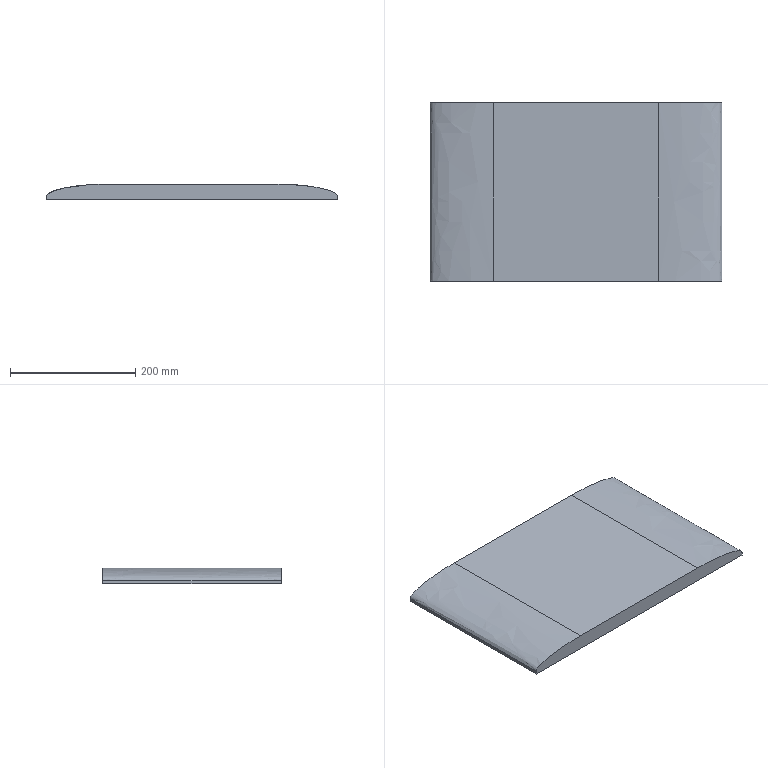Part | SolidWorks | features Fillet 2, Extrusion 1 | 1 solid | 8 faces | box 465 x 285 x 25.029 mm | volume 3079068 mm3 | plane 6 | spline 2
STEP:
#1=CARTESIAN_POINT('',(-232.5,-142.5,5.029));
#2=VERTEX_POINT('',#1);
#3=CARTESIAN_POINT('',(-232.5,-142.5,0.));
#4=VERTEX_POINT('',#3);
#5=CARTESIAN_POINT('',(-232.5,-142.5,25.029));
#6=DIRECTION('',(0.,0.,-1.));
#7=VECTOR('',#6,1000.);
#8=LINE('',#5,#7);
#9=EDGE_CURVE('',#2,#4,#8,.T.);
#10=ORIENTED_EDGE('',*,*,#9,.F.);
#11=CARTESIAN_POINT('',(-232.5,142.5,5.029));
#12=VERTEX_POINT('',#11);
#13=CARTESIAN_POINT('',(-232.5,-142.5,5.029));
#14=CARTESIAN_POINT('',(-232.5,-47.5,5.029));
#15=CARTESIAN_POINT('',(-232.5,47.5,5.029));
#16=CARTESIAN_POINT('',(-232.5,142.5,5.029));
#17=B_SPLINE_CURVE_WITH_KNOTS('',3,(#13,#14,#15,#16),.UNSPECIFIED.,.F.,.F.,(4,4),(0.,1.),.UNSPECIFIED.);
#18=EDGE_CURVE('',#2,#12,#17,.T.);
#19=ORIENTED_EDGE('',*,*,#18,.T.);
#20=CARTESIAN_POINT('',(-232.5,142.5,0.));
#21=VERTEX_POINT('',#20);
#22=CARTESIAN_POINT('',(-232.5,142.5,25.029));
#23=DIRECTION('',(0.,0.,-1.));
#24=VECTOR('',#23,1000.);
#25=LINE('',#22,#24);
#26=EDGE_CURVE('',#12,#21,#25,.T.);
#27=ORIENTED_EDGE('',*,*,#26,.T.);
#28=CARTESIAN_POINT('',(-232.5,-142.5,0.));
#29=DIRECTION('',(0.,-1.,0.));
#30=VECTOR('',#29,1000.);
#31=LINE('',#28,#30);
#32=EDGE_CURVE('',#21,#4,#31,.T.);
#33=ORIENTED_EDGE('',*,*,#32,.T.);
#34=EDGE_LOOP('',(#10,#19,#27,#33));
#35=FACE_OUTER_BOUND('',#34,.T.);
#36=CARTESIAN_POINT('',(-232.5,-142.5,25.029));
#37=DIRECTION('',(1.,0.,0.));
#38=DIRECTION('',(0.,0.,-1.));
#39=AXIS2_PLACEMENT_3D('',#36,#37,#38);
#40=PLANE('',#39);
#41=ADVANCED_FACE('',(#35),#40,.F.);
#42=CARTESIAN_POINT('',(232.5,-142.5,5.029));
#43=VERTEX_POINT('',#42);
#44=CARTESIAN_POINT('',(232.5,-142.5,0.));
#45=VERTEX_POINT('',#44);
#46=CARTESIAN_POINT('',(232.5,-142.5,25.029));
#47=DIRECTION('',(0.,0.,-1.));
#48=VECTOR('',#47,1000.);
#49=LINE('',#46,#48);
#50=EDGE_CURVE('',#43,#45,#49,.T.);
#51=ORIENTED_EDGE('',*,*,#50,.F.);
#52=CARTESIAN_POINT('',(132.5,-142.5,25.029));
#53=VERTEX_POINT('',#52);
#54=CARTESIAN_POINT('',(232.5,-142.5,5.029));
#55=CARTESIAN_POINT('',(232.5,-142.5,5.932));
#56=CARTESIAN_POINT('',(232.05,-142.5,7.274));
#57=CARTESIAN_POINT('',(230.736,-142.5,8.819));
#58=CARTESIAN_POINT('',(229.882,-142.5,9.586));
#59=CARTESIAN_POINT('',(229.405,-142.5,9.968));
#60=CARTESIAN_POINT('',(229.155,-142.5,10.159));
#61=CARTESIAN_POINT('',(229.027,-142.5,10.254));
#62=CARTESIAN_POINT('',(228.962,-142.5,10.302));
#63=CARTESIAN_POINT('',(228.929,-142.5,10.325));
#64=CARTESIAN_POINT('',(228.915,-142.5,10.336));
#65=CARTESIAN_POINT('',(228.906,-142.5,10.342));
#66=CARTESIAN_POINT('',(228.899,-142.5,10.347));
#67=CARTESIAN_POINT('',(228.151,-142.5,10.889));
#68=CARTESIAN_POINT('',(226.869,-142.5,11.687));
#69=CARTESIAN_POINT('',(225.083,-142.5,12.596));
#70=CARTESIAN_POINT('',(224.118,-142.5,13.046));
#71=CARTESIAN_POINT('',(223.618,-142.5,13.269));
#72=CARTESIAN_POINT('',(223.363,-142.5,13.381));
#73=CARTESIAN_POINT('',(223.234,-142.5,13.436));
#74=CARTESIAN_POINT('',(223.17,-142.5,13.464));
#75=CARTESIAN_POINT('',(223.137,-142.5,13.478));
#76=CARTESIAN_POINT('',(223.124,-142.5,13.484));
#77=CARTESIAN_POINT('',(223.114,-142.5,13.488));
#78=CARTESIAN_POINT('',(223.108,-142.5,13.491));
#79=CARTESIAN_POINT('',(221.419,-142.5,14.214));
#80=CARTESIAN_POINT('',(218.59,-142.5,15.259));
#81=CARTESIAN_POINT('',(214.761,-142.5,16.413));
#82=CARTESIAN_POINT('',(212.714,-142.5,16.974));
#83=CARTESIAN_POINT('',(211.658,-142.5,17.251));
#84=CARTESIAN_POINT('',(211.122,-142.5,17.388));
#85=CARTESIAN_POINT('',(210.852,-142.5,17.456));
#86=CARTESIAN_POINT('',(210.716,-142.5,17.49));
#87=CARTESIAN_POINT('',(210.648,-142.5,17.507));
#88=CARTESIAN_POINT('',(210.614,-142.5,17.516));
#89=CARTESIAN_POINT('',(210.599,-142.5,17.519));
#90=CARTESIAN_POINT('',(210.59,-142.5,17.522));
#91=CARTESIAN_POINT('',(210.584,-142.5,17.523));
#92=CARTESIAN_POINT('',(206.95,-142.5,18.432));
#93=CARTESIAN_POINT('',(201.009,-142.5,19.68));
#94=CARTESIAN_POINT('',(193.212,-142.5,20.941));
#95=CARTESIAN_POINT('',(189.096,-142.5,21.522));
#96=CARTESIAN_POINT('',(186.984,-142.5,21.801));
#97=CARTESIAN_POINT('',(185.914,-142.5,21.937));
#98=CARTESIAN_POINT('',(185.376,-142.5,22.004));
#99=CARTESIAN_POINT('',(185.106,-142.5,22.038));
#100=CARTESIAN_POINT('',(184.971,-142.5,22.054));
#101=CARTESIAN_POINT('',(184.903,-142.5,22.063));
#102=CARTESIAN_POINT('',(184.874,-142.5,22.066));
#103=CARTESIAN_POINT('',(184.855,-142.5,22.068));
#104=CARTESIAN_POINT('',(184.843,-142.5,22.07));
#105=CARTESIAN_POINT('',(180.754,-142.5,22.572));
#106=CARTESIAN_POINT('',(174.428,-142.5,23.231));
#107=CARTESIAN_POINT('',(166.692,-142.5,23.834));
#108=CARTESIAN_POINT('',(162.736,-142.5,24.095));
#109=CARTESIAN_POINT('',(160.735,-142.5,24.215));
#110=CARTESIAN_POINT('',(159.729,-142.5,24.273));
#111=CARTESIAN_POINT('',(159.225,-142.5,24.301));
#112=CARTESIAN_POINT('',(158.973,-142.5,24.315));
#113=CARTESIAN_POINT('',(158.846,-142.5,24.322));
#114=CARTESIAN_POINT('',(158.792,-142.5,24.325));
#115=CARTESIAN_POINT('',(158.756,-142.5,24.327));
#116=CARTESIAN_POINT('',(158.737,-142.5,24.328));
#117=CARTESIAN_POINT('',(150.136,-142.5,24.795));
#118=CARTESIAN_POINT('',(141.396,-142.5,25.029));
#119=CARTESIAN_POINT('',(132.5,-142.5,25.029));
#120=B_SPLINE_CURVE_WITH_KNOTS('',3,(#54,#55,#56,#57,#58,#59,#60,#61,#62,#63,#64,#65,#66,#67,#68,#69,#70,#71,#72,#73,#74,#75,#76,#77,#78,#79,#80,#81,#82,#83,#84,#85,#86,#87,#88,#89,#90,#91,#92,#93,#94,#95,#96,#97,#98,#99,#100,#101,#102,#103,#104,#105,#106,#107,#108,#109,#110,#111,#112,#113,#114,#115,#116,#117,#118,#119),.UNSPECIFIED.,.F.,.F.,(4,1,1,1,1,1,1,1,1,2,2,1,1,1,1,1,1,1,1,2,2,1,1,1,1,1,1,1,1,1,2,2,1,1,1,1,1,1,1,1,1,2,2,1,1,1,1,1,1,1,1,2,2,4),(0.,0.03125,0.04687,0.05469,0.05859,0.06055,0.06152,0.06201,0.06226,0.06238,0.0625,0.09375,0.1094,0.1172,0.1211,0.123,0.124,0.1245,0.1248,0.1249,0.125,0.1875,0.2187,0.2344,0.2422,0.2461,0.248,0.249,0.2495,0.2498,0.2499,0.25,0.375,0.4375,0.4687,0.4844,0.4922,0.4961,0.498,0.499,0.4995,0.4998,0.5,0.625,0.6875,0.7187,0.7344,0.7422,0.7461,0.748,0.749,0.7495,0.75,1.),.UNSPECIFIED.);
#121=EDGE_CURVE('',#43,#53,#120,.T.);
#122=ORIENTED_EDGE('',*,*,#121,.T.);
#123=CARTESIAN_POINT('',(-132.5,-142.5,25.029));
#124=VERTEX_POINT('',#123);
#125=CARTESIAN_POINT('',(232.5,-142.5,25.029));
#126=DIRECTION('',(1.,0.,0.));
#127=VECTOR('',#126,1000.);
#128=LINE('',#125,#127);
#129=EDGE_CURVE('',#124,#53,#128,.T.);
#130=ORIENTED_EDGE('',*,*,#129,.F.);
#131=CARTESIAN_POINT('',(-132.5,-142.5,25.029));
#132=CARTESIAN_POINT('',(-136.95,-142.5,25.029));
#133=CARTESIAN_POINT('',(-143.567,-142.5,24.941));
#134=CARTESIAN_POINT('',(-151.185,-142.5,24.686));
#135=CARTESIAN_POINT('',(-154.968,-142.5,24.52));
#136=CARTESIAN_POINT('',(-156.853,-142.5,24.427));
#137=CARTESIAN_POINT('',(-157.794,-142.5,24.378));
#138=CARTESIAN_POINT('',(-158.264,-142.5,24.353));
#139=CARTESIAN_POINT('',(-158.499,-142.5,24.341));
#140=CARTESIAN_POINT('',(-158.616,-142.5,24.334));
#141=CARTESIAN_POINT('',(-158.667,-142.5,24.332));
#142=CARTESIAN_POINT('',(-158.7,-142.5,24.33));
#143=CARTESIAN_POINT('',(-158.716,-142.5,24.329));
#144=CARTESIAN_POINT('',(-163.364,-142.5,24.076));
#145=CARTESIAN_POINT('',(-170.105,-142.5,23.605));
#146=CARTESIAN_POINT('',(-177.613,-142.5,22.89));
#147=CARTESIAN_POINT('',(-181.279,-142.5,22.491));
#148=CARTESIAN_POINT('',(-183.089,-142.5,22.281));
#149=CARTESIAN_POINT('',(-183.989,-142.5,22.174));
#150=CARTESIAN_POINT('',(-184.437,-142.5,22.12));
#151=CARTESIAN_POINT('',(-184.661,-142.5,22.092));
#152=CARTESIAN_POINT('',(-184.773,-142.5,22.079));
#153=CARTESIAN_POINT('',(-184.829,-142.5,22.072));
#154=CARTESIAN_POINT('',(-184.853,-142.5,22.069));
#155=CARTESIAN_POINT('',(-184.869,-142.5,22.067));
#156=CARTESIAN_POINT('',(-184.875,-142.5,22.066));
#157=CARTESIAN_POINT('',(-189.859,-142.5,21.453));
#158=CARTESIAN_POINT('',(-196.82,-142.5,20.422));
#159=CARTESIAN_POINT('',(-204.065,-142.5,19.021));
#160=CARTESIAN_POINT('',(-207.468,-142.5,18.271));
#161=CARTESIAN_POINT('',(-209.114,-142.5,17.884));
#162=CARTESIAN_POINT('',(-209.924,-142.5,17.687));
#163=CARTESIAN_POINT('',(-210.325,-142.5,17.588));
#164=CARTESIAN_POINT('',(-210.525,-142.5,17.538));
#165=CARTESIAN_POINT('',(-210.625,-142.5,17.513));
#166=CARTESIAN_POINT('',(-210.675,-142.5,17.5));
#167=CARTESIAN_POINT('',(-210.7,-142.5,17.494));
#168=CARTESIAN_POINT('',(-210.71,-142.5,17.492));
#169=CARTESIAN_POINT('',(-210.717,-142.5,17.49));
#170=CARTESIAN_POINT('',(-210.72,-142.5,17.489));
#171=CARTESIAN_POINT('',(-213.209,-142.5,16.864));
#172=CARTESIAN_POINT('',(-216.634,-142.5,15.891));
#173=CARTESIAN_POINT('',(-220.101,-142.5,14.69));
#174=CARTESIAN_POINT('',(-221.702,-142.5,14.073));
#175=CARTESIAN_POINT('',(-222.469,-142.5,13.76));
#176=CARTESIAN_POINT('',(-222.845,-142.5,13.603));
#177=CARTESIAN_POINT('',(-223.031,-142.5,13.524));
#178=CARTESIAN_POINT('',(-223.123,-142.5,13.484));
#179=CARTESIAN_POINT('',(-223.169,-142.5,13.465));
#180=CARTESIAN_POINT('',(-223.192,-142.5,13.455));
#181=CARTESIAN_POINT('',(-223.202,-142.5,13.45));
#182=CARTESIAN_POINT('',(-223.208,-142.5,13.448));
#183=CARTESIAN_POINT('',(-223.21,-142.5,13.447));
#184=CARTESIAN_POINT('',(-224.392,-142.5,12.937));
#185=CARTESIAN_POINT('',(-225.993,-142.5,12.164));
#186=CARTESIAN_POINT('',(-227.572,-142.5,11.241));
#187=CARTESIAN_POINT('',(-228.29,-142.5,10.774));
#188=CARTESIAN_POINT('',(-228.631,-142.5,10.539));
#189=CARTESIAN_POINT('',(-228.797,-142.5,10.421));
#190=CARTESIAN_POINT('',(-228.879,-142.5,10.362));
#191=CARTESIAN_POINT('',(-228.919,-142.5,10.333));
#192=CARTESIAN_POINT('',(-228.94,-142.5,10.318));
#193=CARTESIAN_POINT('',(-228.948,-142.5,10.312));
#194=CARTESIAN_POINT('',(-228.954,-142.5,10.307));
#195=CARTESIAN_POINT('',(-228.955,-142.5,10.306));
#196=CARTESIAN_POINT('',(-231.32,-142.5,8.577));
#197=CARTESIAN_POINT('',(-232.5,-142.5,6.819));
#198=CARTESIAN_POINT('',(-232.5,-142.5,5.029));
#199=B_SPLINE_CURVE_WITH_KNOTS('',3,(#131,#132,#133,#134,#135,#136,#137,#138,#139,#140,#141,#142,#143,#144,#145,#146,#147,#148,#149,#150,#151,#152,#153,#154,#155,#156,#157,#158,#159,#160,#161,#162,#163,#164,#165,#166,#167,#168,#169,#170,#171,#172,#173,#174,#175,#176,#177,#178,#179,#180,#181,#182,#183,#184,#185,#186,#187,#188,#189,#190,#191,#192,#193,#194,#195,#196,#197,#198),.UNSPECIFIED.,.F.,.F.,(4,1,1,1,1,1,1,1,1,2,2,1,1,1,1,1,1,1,1,1,2,2,1,1,1,1,1,1,1,1,1,1,2,2,1,1,1,1,1,1,1,1,1,2,2,1,1,1,1,1,1,1,1,2,2,4),(0.,0.125,0.1875,0.2188,0.2344,0.2422,0.2461,0.248,0.249,0.2495,0.25,0.375,0.4375,0.4688,0.4844,0.4922,0.4961,0.498,0.499,0.4995,0.4998,0.5,0.625,0.6875,0.7188,0.7344,0.7422,0.7461,0.748,0.749,0.7495,0.7498,0.7499,0.75,0.8125,0.8438,0.8594,0.8672,0.8711,0.873,0.874,0.8745,0.8748,0.8749,0.875,0.9063,0.9219,0.9297,0.9336,0.9355,0.9365,0.937,0.9373,0.9374,0.9375,1.),.UNSPECIFIED.);
#200=EDGE_CURVE('',#124,#2,#199,.T.);
#201=ORIENTED_EDGE('',*,*,#200,.T.);
#202=ORIENTED_EDGE('',*,*,#9,.T.);
#203=CARTESIAN_POINT('',(232.5,-142.5,0.));
#204=DIRECTION('',(1.,0.,0.));
#205=VECTOR('',#204,1000.);
#206=LINE('',#203,#205);
#207=EDGE_CURVE('',#4,#45,#206,.T.);
#208=ORIENTED_EDGE('',*,*,#207,.T.);
#209=EDGE_LOOP('',(#51,#122,#130,#201,#202,#208));
#210=FACE_OUTER_BOUND('',#209,.T.);
#211=CARTESIAN_POINT('',(232.5,-142.5,25.029));
#212=DIRECTION('',(0.,1.,0.));
#213=DIRECTION('',(-1.,0.,0.));
#214=AXIS2_PLACEMENT_3D('',#211,#212,#213);
#215=PLANE('',#214);
#216=ADVANCED_FACE('',(#210),#215,.F.);
#217=CARTESIAN_POINT('',(232.5,142.5,5.029));
#218=VERTEX_POINT('',#217);
#219=CARTESIAN_POINT('',(232.5,142.5,0.));
#220=VERTEX_POINT('',#219);
#221=CARTESIAN_POINT('',(232.5,142.5,25.029));
#222=DIRECTION('',(0.,0.,-1.));
#223=VECTOR('',#222,1000.);
#224=LINE('',#221,#223);
#225=EDGE_CURVE('',#218,#220,#224,.T.);
#226=ORIENTED_EDGE('',*,*,#225,.F.);
#227=CARTESIAN_POINT('',(232.5,142.5,5.029));
#228=CARTESIAN_POINT('',(232.5,47.5,5.029));
#229=CARTESIAN_POINT('',(232.5,-47.5,5.029));
#230=CARTESIAN_POINT('',(232.5,-142.5,5.029));
#231=B_SPLINE_CURVE_WITH_KNOTS('',3,(#227,#228,#229,#230),.UNSPECIFIED.,.F.,.F.,(4,4),(0.,1.),.UNSPECIFIED.);
#232=EDGE_CURVE('',#218,#43,#231,.T.);
#233=ORIENTED_EDGE('',*,*,#232,.T.);
#234=ORIENTED_EDGE('',*,*,#50,.T.);
#235=CARTESIAN_POINT('',(232.5,-142.5,0.));
#236=DIRECTION('',(0.,1.,0.));
#237=VECTOR('',#236,1000.);
#238=LINE('',#235,#237);
#239=EDGE_CURVE('',#45,#220,#238,.T.);
#240=ORIENTED_EDGE('',*,*,#239,.T.);
#241=EDGE_LOOP('',(#226,#233,#234,#240));
#242=FACE_OUTER_BOUND('',#241,.T.);
#243=CARTESIAN_POINT('',(232.5,-142.5,25.029));
#244=DIRECTION('',(-1.,0.,0.));
#245=DIRECTION('',(0.,0.,1.));
#246=AXIS2_PLACEMENT_3D('',#243,#244,#245);
#247=PLANE('',#246);
#248=ADVANCED_FACE('',(#242),#247,.F.);
#249=CARTESIAN_POINT('',(132.5,142.5,25.029));
#250=VERTEX_POINT('',#249);
#251=CARTESIAN_POINT('',(-132.5,142.5,25.029));
#252=VERTEX_POINT('',#251);
#253=CARTESIAN_POINT('',(232.5,142.5,25.029));
#254=DIRECTION('',(-1.,0.,0.));
#255=VECTOR('',#254,1000.);
#256=LINE('',#253,#255);
#257=EDGE_CURVE('',#250,#252,#256,.T.);
#258=ORIENTED_EDGE('',*,*,#257,.F.);
#259=CARTESIAN_POINT('',(132.5,142.5,25.029));
#260=CARTESIAN_POINT('',(136.95,142.5,25.029));
#261=CARTESIAN_POINT('',(143.567,142.5,24.941));
#262=CARTESIAN_POINT('',(151.185,142.5,24.686));
#263=CARTESIAN_POINT('',(154.968,142.5,24.52));
#264=CARTESIAN_POINT('',(156.853,142.5,24.427));
#265=CARTESIAN_POINT('',(157.794,142.5,24.378));
#266=CARTESIAN_POINT('',(158.264,142.5,24.353));
#267=CARTESIAN_POINT('',(158.499,142.5,24.341));
#268=CARTESIAN_POINT('',(158.616,142.5,24.334));
#269=CARTESIAN_POINT('',(158.667,142.5,24.332));
#270=CARTESIAN_POINT('',(158.7,142.5,24.33));
#271=CARTESIAN_POINT('',(158.716,142.5,24.329));
#272=CARTESIAN_POINT('',(163.364,142.5,24.076));
#273=CARTESIAN_POINT('',(170.105,142.5,23.605));
#274=CARTESIAN_POINT('',(177.613,142.5,22.89));
#275=CARTESIAN_POINT('',(181.279,142.5,22.491));
#276=CARTESIAN_POINT('',(183.089,142.5,22.281));
#277=CARTESIAN_POINT('',(183.989,142.5,22.174));
#278=CARTESIAN_POINT('',(184.437,142.5,22.12));
#279=CARTESIAN_POINT('',(184.661,142.5,22.092));
#280=CARTESIAN_POINT('',(184.773,142.5,22.079));
#281=CARTESIAN_POINT('',(184.829,142.5,22.072));
#282=CARTESIAN_POINT('',(184.853,142.5,22.069));
#283=CARTESIAN_POINT('',(184.869,142.5,22.067));
#284=CARTESIAN_POINT('',(184.875,142.5,22.066));
#285=CARTESIAN_POINT('',(189.859,142.5,21.453));
#286=CARTESIAN_POINT('',(196.82,142.5,20.422));
#287=CARTESIAN_POINT('',(204.065,142.5,19.021));
#288=CARTESIAN_POINT('',(207.468,142.5,18.271));
#289=CARTESIAN_POINT('',(209.114,142.5,17.884));
#290=CARTESIAN_POINT('',(209.924,142.5,17.687));
#291=CARTESIAN_POINT('',(210.325,142.5,17.588));
#292=CARTESIAN_POINT('',(210.525,142.5,17.538));
#293=CARTESIAN_POINT('',(210.625,142.5,17.513));
#294=CARTESIAN_POINT('',(210.675,142.5,17.5));
#295=CARTESIAN_POINT('',(210.7,142.5,17.494));
#296=CARTESIAN_POINT('',(210.71,142.5,17.492));
#297=CARTESIAN_POINT('',(210.717,142.5,17.49));
#298=CARTESIAN_POINT('',(210.72,142.5,17.489));
#299=CARTESIAN_POINT('',(213.209,142.5,16.864));
#300=CARTESIAN_POINT('',(216.634,142.5,15.891));
#301=CARTESIAN_POINT('',(220.101,142.5,14.69));
#302=CARTESIAN_POINT('',(221.702,142.5,14.073));
#303=CARTESIAN_POINT('',(222.469,142.5,13.76));
#304=CARTESIAN_POINT('',(222.845,142.5,13.603));
#305=CARTESIAN_POINT('',(223.031,142.5,13.524));
#306=CARTESIAN_POINT('',(223.123,142.5,13.484));
#307=CARTESIAN_POINT('',(223.169,142.5,13.465));
#308=CARTESIAN_POINT('',(223.192,142.5,13.455));
#309=CARTESIAN_POINT('',(223.202,142.5,13.45));
#310=CARTESIAN_POINT('',(223.208,142.5,13.448));
#311=CARTESIAN_POINT('',(223.21,142.5,13.447));
#312=CARTESIAN_POINT('',(224.392,142.5,12.937));
#313=CARTESIAN_POINT('',(225.993,142.5,12.164));
#314=CARTESIAN_POINT('',(227.572,142.5,11.241));
#315=CARTESIAN_POINT('',(228.29,142.5,10.774));
#316=CARTESIAN_POINT('',(228.631,142.5,10.539));
#317=CARTESIAN_POINT('',(228.797,142.5,10.421));
#318=CARTESIAN_POINT('',(228.879,142.5,10.362));
#319=CARTESIAN_POINT('',(228.919,142.5,10.333));
#320=CARTESIAN_POINT('',(228.94,142.5,10.318));
#321=CARTESIAN_POINT('',(228.948,142.5,10.312));
#322=CARTESIAN_POINT('',(228.954,142.5,10.307));
#323=CARTESIAN_POINT('',(228.955,142.5,10.306));
#324=CARTESIAN_POINT('',(231.32,142.5,8.577));
#325=CARTESIAN_POINT('',(232.5,142.5,6.819));
#326=CARTESIAN_POINT('',(232.5,142.5,5.029));
#327=B_SPLINE_CURVE_WITH_KNOTS('',3,(#259,#260,#261,#262,#263,#264,#265,#266,#267,#268,#269,#270,#271,#272,#273,#274,#275,#276,#277,#278,#279,#280,#281,#282,#283,#284,#285,#286,#287,#288,#289,#290,#291,#292,#293,#294,#295,#296,#297,#298,#299,#300,#301,#302,#303,#304,#305,#306,#307,#308,#309,#310,#311,#312,#313,#314,#315,#316,#317,#318,#319,#320,#321,#322,#323,#324,#325,#326),.UNSPECIFIED.,.F.,.F.,(4,1,1,1,1,1,1,1,1,2,2,1,1,1,1,1,1,1,1,1,2,2,1,1,1,1,1,1,1,1,1,1,2,2,1,1,1,1,1,1,1,1,1,2,2,1,1,1,1,1,1,1,1,2,2,4),(0.,0.125,0.1875,0.2187,0.2344,0.2422,0.2461,0.248,0.249,0.2495,0.25,0.375,0.4375,0.4687,0.4844,0.4922,0.4961,0.498,0.499,0.4995,0.4998,0.5,0.625,0.6875,0.7187,0.7344,0.7422,0.7461,0.748,0.749,0.7495,0.7498,0.7499,0.75,0.8125,0.8437,0.8594,0.8672,0.8711,0.873,0.874,0.8745,0.8748,0.8749,0.875,0.9062,0.9219,0.9297,0.9336,0.9355,0.9365,0.937,0.9373,0.9374,0.9375,1.),.UNSPECIFIED.);
#328=EDGE_CURVE('',#250,#218,#327,.T.);
#329=ORIENTED_EDGE('',*,*,#328,.T.);
#330=ORIENTED_EDGE('',*,*,#225,.T.);
#331=CARTESIAN_POINT('',(232.5,142.5,0.));
#332=DIRECTION('',(-1.,0.,0.));
#333=VECTOR('',#332,1000.);
#334=LINE('',#331,#333);
#335=EDGE_CURVE('',#220,#21,#334,.T.);
#336=ORIENTED_EDGE('',*,*,#335,.T.);
#337=ORIENTED_EDGE('',*,*,#26,.F.);
#338=CARTESIAN_POINT('',(-232.5,142.5,5.029));
#339=CARTESIAN_POINT('',(-232.5,142.5,5.932));
#340=CARTESIAN_POINT('',(-232.05,142.5,7.274));
#341=CARTESIAN_POINT('',(-230.736,142.5,8.819));
#342=CARTESIAN_POINT('',(-229.882,142.5,9.586));
#343=CARTESIAN_POINT('',(-229.405,142.5,9.968));
#344=CARTESIAN_POINT('',(-229.155,142.5,10.159));
#345=CARTESIAN_POINT('',(-229.027,142.5,10.254));
#346=CARTESIAN_POINT('',(-228.962,142.5,10.302));
#347=CARTESIAN_POINT('',(-228.929,142.5,10.325));
#348=CARTESIAN_POINT('',(-228.915,142.5,10.336));
#349=CARTESIAN_POINT('',(-228.906,142.5,10.342));
#350=CARTESIAN_POINT('',(-228.899,142.5,10.347));
#351=CARTESIAN_POINT('',(-228.151,142.5,10.889));
#352=CARTESIAN_POINT('',(-226.869,142.5,11.687));
#353=CARTESIAN_POINT('',(-225.083,142.5,12.596));
#354=CARTESIAN_POINT('',(-224.118,142.5,13.046));
#355=CARTESIAN_POINT('',(-223.618,142.5,13.269));
#356=CARTESIAN_POINT('',(-223.363,142.5,13.381));
#357=CARTESIAN_POINT('',(-223.234,142.5,13.436));
#358=CARTESIAN_POINT('',(-223.17,142.5,13.464));
#359=CARTESIAN_POINT('',(-223.137,142.5,13.478));
#360=CARTESIAN_POINT('',(-223.124,142.5,13.484));
#361=CARTESIAN_POINT('',(-223.114,142.5,13.488));
#362=CARTESIAN_POINT('',(-223.108,142.5,13.491));
#363=CARTESIAN_POINT('',(-221.419,142.5,14.214));
#364=CARTESIAN_POINT('',(-218.59,142.5,15.259));
#365=CARTESIAN_POINT('',(-214.761,142.5,16.413));
#366=CARTESIAN_POINT('',(-212.714,142.5,16.974));
#367=CARTESIAN_POINT('',(-211.658,142.5,17.251));
#368=CARTESIAN_POINT('',(-211.122,142.5,17.388));
#369=CARTESIAN_POINT('',(-210.852,142.5,17.456));
#370=CARTESIAN_POINT('',(-210.716,142.5,17.49));
#371=CARTESIAN_POINT('',(-210.648,142.5,17.507));
#372=CARTESIAN_POINT('',(-210.614,142.5,17.516));
#373=CARTESIAN_POINT('',(-210.599,142.5,17.519));
#374=CARTESIAN_POINT('',(-210.59,142.5,17.522));
#375=CARTESIAN_POINT('',(-210.584,142.5,17.523));
#376=CARTESIAN_POINT('',(-206.95,142.5,18.432));
#377=CARTESIAN_POINT('',(-201.009,142.5,19.68));
#378=CARTESIAN_POINT('',(-193.212,142.5,20.941));
#379=CARTESIAN_POINT('',(-189.096,142.5,21.522));
#380=CARTESIAN_POINT('',(-186.984,142.5,21.801));
#381=CARTESIAN_POINT('',(-185.914,142.5,21.937));
#382=CARTESIAN_POINT('',(-185.376,142.5,22.004));
#383=CARTESIAN_POINT('',(-185.106,142.5,22.038));
#384=CARTESIAN_POINT('',(-184.971,142.5,22.054));
#385=CARTESIAN_POINT('',(-184.903,142.5,22.063));
#386=CARTESIAN_POINT('',(-184.874,142.5,22.066));
#387=CARTESIAN_POINT('',(-184.855,142.5,22.068));
#388=CARTESIAN_POINT('',(-184.843,142.5,22.07));
#389=CARTESIAN_POINT('',(-180.754,142.5,22.572));
#390=CARTESIAN_POINT('',(-174.428,142.5,23.231));
#391=CARTESIAN_POINT('',(-166.692,142.5,23.834));
#392=CARTESIAN_POINT('',(-162.736,142.5,24.095));
#393=CARTESIAN_POINT('',(-160.735,142.5,24.215));
#394=CARTESIAN_POINT('',(-159.729,142.5,24.273));
#395=CARTESIAN_POINT('',(-159.225,142.5,24.301));
#396=CARTESIAN_POINT('',(-158.973,142.5,24.315));
#397=CARTESIAN_POINT('',(-158.846,142.5,24.322));
#398=CARTESIAN_POINT('',(-158.792,142.5,24.325));
#399=CARTESIAN_POINT('',(-158.756,142.5,24.327));
#400=CARTESIAN_POINT('',(-158.737,142.5,24.328));
#401=CARTESIAN_POINT('',(-150.136,142.5,24.795));
#402=CARTESIAN_POINT('',(-141.396,142.5,25.029));
#403=CARTESIAN_POINT('',(-132.5,142.5,25.029));
#404=B_SPLINE_CURVE_WITH_KNOTS('',3,(#338,#339,#340,#341,#342,#343,#344,#345,#346,#347,#348,#349,#350,#351,#352,#353,#354,#355,#356,#357,#358,#359,#360,#361,#362,#363,#364,#365,#366,#367,#368,#369,#370,#371,#372,#373,#374,#375,#376,#377,#378,#379,#380,#381,#382,#383,#384,#385,#386,#387,#388,#389,#390,#391,#392,#393,#394,#395,#396,#397,#398,#399,#400,#401,#402,#403),.UNSPECIFIED.,.F.,.F.,(4,1,1,1,1,1,1,1,1,2,2,1,1,1,1,1,1,1,1,2,2,1,1,1,1,1,1,1,1,1,2,2,1,1,1,1,1,1,1,1,1,2,2,1,1,1,1,1,1,1,1,2,2,4),(0.,0.03125,0.04688,0.05469,0.05859,0.06055,0.06152,0.06201,0.06226,0.06238,0.0625,0.09375,0.1094,0.1172,0.1211,0.123,0.124,0.1245,0.1248,0.1249,0.125,0.1875,0.2187,0.2344,0.2422,0.2461,0.248,0.249,0.2495,0.2498,0.2499,0.25,0.375,0.4375,0.4687,0.4844,0.4922,0.4961,0.498,0.499,0.4995,0.4998,0.5,0.625,0.6875,0.7187,0.7344,0.7422,0.7461,0.748,0.749,0.7495,0.75,1.),.UNSPECIFIED.);
#405=EDGE_CURVE('',#12,#252,#404,.T.);
#406=ORIENTED_EDGE('',*,*,#405,.T.);
#407=EDGE_LOOP('',(#258,#329,#330,#336,#337,#406));
#408=FACE_OUTER_BOUND('',#407,.T.);
#409=CARTESIAN_POINT('',(232.5,142.5,25.029));
#410=DIRECTION('',(0.,-1.,0.));
#411=DIRECTION('',(1.,0.,0.));
#412=AXIS2_PLACEMENT_3D('',#409,#410,#411);
#413=PLANE('',#412);
#414=ADVANCED_FACE('',(#408),#413,.F.);
#415=ORIENTED_EDGE('',*,*,#129,.T.);
#416=CARTESIAN_POINT('',(132.5,-142.5,25.029));
#417=CARTESIAN_POINT('',(132.5,-47.5,25.029));
#418=CARTESIAN_POINT('',(132.5,47.5,25.029));
#419=CARTESIAN_POINT('',(132.5,142.5,25.029));
#420=B_SPLINE_CURVE_WITH_KNOTS('',3,(#416,#417,#418,#419),.UNSPECIFIED.,.F.,.F.,(4,4),(0.,1.),.UNSPECIFIED.);
#421=EDGE_CURVE('',#53,#250,#420,.T.);
#422=ORIENTED_EDGE('',*,*,#421,.T.);
#423=ORIENTED_EDGE('',*,*,#257,.T.);
#424=CARTESIAN_POINT('',(-132.5,142.5,25.029));
#425=CARTESIAN_POINT('',(-132.5,47.5,25.029));
#426=CARTESIAN_POINT('',(-132.5,-47.5,25.029));
#427=CARTESIAN_POINT('',(-132.5,-142.5,25.029));
#428=B_SPLINE_CURVE_WITH_KNOTS('',3,(#424,#425,#426,#427),.UNSPECIFIED.,.F.,.F.,(4,4),(0.,1.),.UNSPECIFIED.);
#429=EDGE_CURVE('',#252,#124,#428,.T.);
#430=ORIENTED_EDGE('',*,*,#429,.T.);
#431=EDGE_LOOP('',(#415,#422,#423,#430));
#432=FACE_OUTER_BOUND('',#431,.T.);
#433=CARTESIAN_POINT('',(0.,0.,25.029));
#434=DIRECTION('',(0.,0.,1.));
#435=DIRECTION('',(1.,0.,0.));
#436=AXIS2_PLACEMENT_3D('',#433,#434,#435);
#437=PLANE('',#436);
#438=ADVANCED_FACE('',(#432),#437,.T.);
#439=ORIENTED_EDGE('',*,*,#32,.F.);
#440=ORIENTED_EDGE('',*,*,#335,.F.);
#441=ORIENTED_EDGE('',*,*,#239,.F.);
#442=ORIENTED_EDGE('',*,*,#207,.F.);
#443=EDGE_LOOP('',(#439,#440,#441,#442));
#444=FACE_OUTER_BOUND('',#443,.T.);
#445=CARTESIAN_POINT('',(0.,0.,0.));
#446=DIRECTION('',(0.,0.,1.));
#447=DIRECTION('',(1.,0.,0.));
#448=AXIS2_PLACEMENT_3D('',#445,#446,#447);
#449=PLANE('',#448);
#450=ADVANCED_FACE('',(#444),#449,.F.);
#451=ORIENTED_EDGE('',*,*,#405,.F.);
#452=ORIENTED_EDGE('',*,*,#18,.F.);
#453=ORIENTED_EDGE('',*,*,#200,.F.);
#454=ORIENTED_EDGE('',*,*,#429,.F.);
#455=EDGE_LOOP('',(#451,#452,#453,#454));
#456=FACE_OUTER_BOUND('',#455,.T.);
#457=CARTESIAN_POINT('',(-232.5,-156.75,5.029));
#458=CARTESIAN_POINT('',(-232.5,-52.25,5.029));
#459=CARTESIAN_POINT('',(-232.5,52.25,5.029));
#460=CARTESIAN_POINT('',(-232.5,156.75,5.029));
#461=CARTESIAN_POINT('',(-232.5,-156.75,25.029));
#462=CARTESIAN_POINT('',(-232.5,-52.25,25.029));
#463=CARTESIAN_POINT('',(-232.5,52.25,25.029));
#464=CARTESIAN_POINT('',(-232.5,156.75,25.029));
#465=CARTESIAN_POINT('',(-132.5,-156.75,25.029));
#466=CARTESIAN_POINT('',(-132.5,-52.25,25.029));
#467=CARTESIAN_POINT('',(-132.5,52.25,25.029));
#468=CARTESIAN_POINT('',(-132.5,156.75,25.029));
#469=(BOUNDED_SURFACE()B_SPLINE_SURFACE(2,3,((#457,#458,#459,#460),(#461,#462,#463,#464),(#465,#466,#467,#468)),.UNSPECIFIED.,.F.,.F.,.F.)B_SPLINE_SURFACE_WITH_KNOTS((3,3),(4,4),(0.,1.),(-0.1568,0.1567),.UNSPECIFIED.)GEOMETRIC_REPRESENTATION_ITEM()RATIONAL_B_SPLINE_SURFACE(((1.,1.,1.,1.),(0.7071,0.7071,0.7071,0.7071),(1.,1.,1.,1.)))REPRESENTATION_ITEM('')SURFACE());
#470=ADVANCED_FACE('',(#456),#469,.T.);
#471=ORIENTED_EDGE('',*,*,#121,.F.);
#472=ORIENTED_EDGE('',*,*,#232,.F.);
#473=ORIENTED_EDGE('',*,*,#328,.F.);
#474=ORIENTED_EDGE('',*,*,#421,.F.);
#475=EDGE_LOOP('',(#471,#472,#473,#474));
#476=FACE_OUTER_BOUND('',#475,.T.);
#477=CARTESIAN_POINT('',(232.5,156.75,5.029));
#478=CARTESIAN_POINT('',(232.5,52.25,5.029));
#479=CARTESIAN_POINT('',(232.5,-52.25,5.029));
#480=CARTESIAN_POINT('',(232.5,-156.75,5.029));
#481=CARTESIAN_POINT('',(232.5,156.75,25.029));
#482=CARTESIAN_POINT('',(232.5,52.25,25.029));
#483=CARTESIAN_POINT('',(232.5,-52.25,25.029));
#484=CARTESIAN_POINT('',(232.5,-156.75,25.029));
#485=CARTESIAN_POINT('',(132.5,156.75,25.029));
#486=CARTESIAN_POINT('',(132.5,52.25,25.029));
#487=CARTESIAN_POINT('',(132.5,-52.25,25.029));
#488=CARTESIAN_POINT('',(132.5,-156.75,25.029));
#489=(BOUNDED_SURFACE()B_SPLINE_SURFACE(2,3,((#477,#478,#479,#480),(#481,#482,#483,#484),(#485,#486,#487,#488)),.UNSPECIFIED.,.F.,.F.,.F.)B_SPLINE_SURFACE_WITH_KNOTS((3,3),(4,4),(0.,1.),(-0.1568,0.1568),.UNSPECIFIED.)GEOMETRIC_REPRESENTATION_ITEM()RATIONAL_B_SPLINE_SURFACE(((1.,1.,1.,1.),(0.7071,0.7071,0.7071,0.7071),(1.,1.,1.,1.)))REPRESENTATION_ITEM('')SURFACE());
#490=ADVANCED_FACE('',(#476),#489,.T.);
#491=CLOSED_SHELL('',(#41,#216,#248,#414,#438,#450,#470,#490));
#492=MANIFOLD_SOLID_BREP('',#491);
#493=CARTESIAN_POINT('',(0.,0.,0.));
#494=DIRECTION('',(0.,0.,1.));
#495=DIRECTION('',(1.,0.,0.));
#496=AXIS2_PLACEMENT_3D('',#493,#494,#495);
#497=(LENGTH_UNIT()NAMED_UNIT(*)SI_UNIT(.MILLI.,.METRE.));
#498=UNCERTAINTY_MEASURE_WITH_UNIT(LENGTH_MEASURE(0.00001),#497,'','');
#499=(NAMED_UNIT(*)PLANE_ANGLE_UNIT()SI_UNIT($,.RADIAN.));
#500=(NAMED_UNIT(*)SI_UNIT($,.STERADIAN.)SOLID_ANGLE_UNIT());
#501=(GEOMETRIC_REPRESENTATION_CONTEXT(3)GLOBAL_UNCERTAINTY_ASSIGNED_CONTEXT((#498))GLOBAL_UNIT_ASSIGNED_CONTEXT((#497,#499,#500))REPRESENTATION_CONTEXT('',''));
#502=ADVANCED_BREP_SHAPE_REPRESENTATION('',(#492,#496),#501);